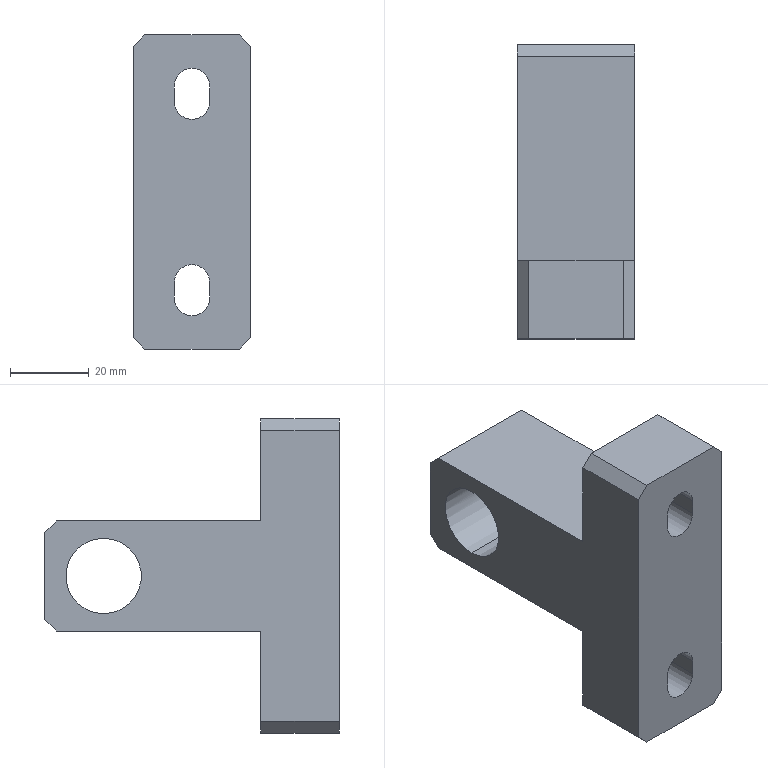Part | STEP file | 13-Guardrail bracket | 1 solid | 42 faces | box 30 x 75 x 80 mm | volume 78230 mm3 | plane 26 | cylinder 16 | commonest cylinder face diameters 9 x6 15 x6 6.8 x2 19.2 x2